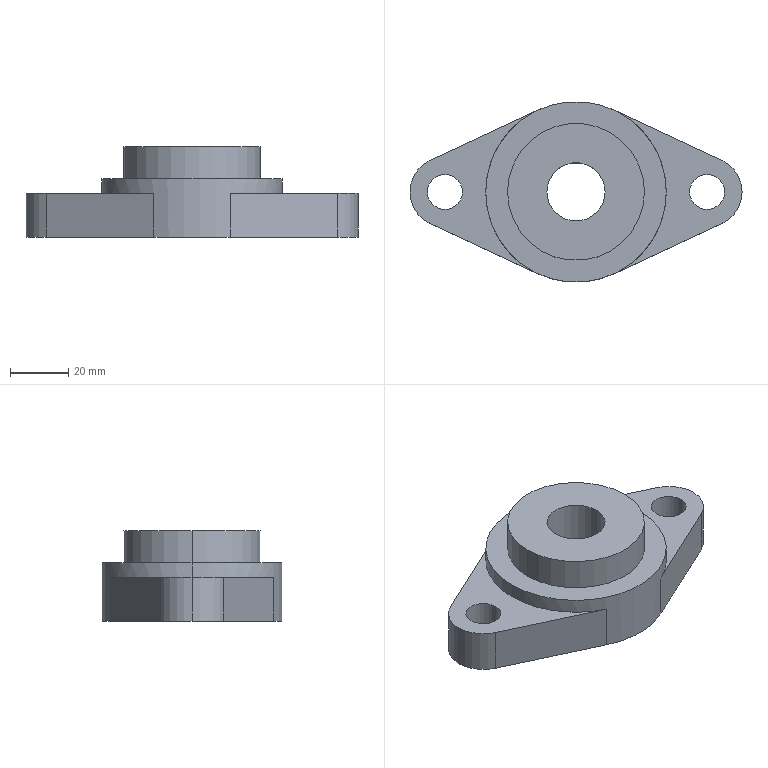Part | STEP file | Bearing housing 2 | 1 solid | 22 faces | box 114 x 62 x 31 mm | volume 91139 mm3 | cylinder 13 | plane 9 | commonest cylinder face diameters 12 x4 24 x3 20 x2 47 x2 62 x2
STEP:
#1=CARTESIAN_POINT('',(-89.013,-0.9655,15.));
#2=VERTEX_POINT('',#1);
#3=CARTESIAN_POINT('',(-101.013,-0.9655,15.));
#4=VERTEX_POINT('',#3);
#5=CARTESIAN_POINT('',(-95.013,-0.9655,15.));
#6=DIRECTION('',(0.,0.,-1.));
#7=DIRECTION('',(-1.,0.,0.));
#8=AXIS2_PLACEMENT_3D('',#5,#6,#7);
#9=CIRCLE('',#8,6.);
#10=EDGE_CURVE('',#2,#4,#9,.T.);
#11=ORIENTED_EDGE('',*,*,#10,.F.);
#12=CARTESIAN_POINT('',(-89.013,-0.9655,0.));
#13=VERTEX_POINT('',#12);
#14=CARTESIAN_POINT('',(-89.013,-0.9655,15.));
#15=DIRECTION('',(0.,0.,-1.));
#16=VECTOR('',#15,1000.);
#17=LINE('',#14,#16);
#18=EDGE_CURVE('',#2,#13,#17,.T.);
#19=ORIENTED_EDGE('',*,*,#18,.T.);
#20=CARTESIAN_POINT('',(-101.013,-0.9655,0.));
#21=VERTEX_POINT('',#20);
#22=CARTESIAN_POINT('',(-95.013,-0.9655,0.));
#23=DIRECTION('',(0.,0.,-1.));
#24=DIRECTION('',(-1.,0.,0.));
#25=AXIS2_PLACEMENT_3D('',#22,#23,#24);
#26=CIRCLE('',#25,6.);
#27=EDGE_CURVE('',#13,#21,#26,.T.);
#28=ORIENTED_EDGE('',*,*,#27,.T.);
#29=CARTESIAN_POINT('',(-101.013,-0.9655,15.));
#30=DIRECTION('',(0.,0.,-1.));
#31=VECTOR('',#30,1000.);
#32=LINE('',#29,#31);
#33=EDGE_CURVE('',#4,#21,#32,.T.);
#34=ORIENTED_EDGE('',*,*,#33,.F.);
#35=EDGE_LOOP('',(#11,#19,#28,#34));
#36=FACE_OUTER_BOUND('',#35,.T.);
#37=CARTESIAN_POINT('',(-95.013,-0.9655,15.));
#38=DIRECTION('',(0.,0.,-1.));
#39=DIRECTION('',(-1.,0.,0.));
#40=AXIS2_PLACEMENT_3D('',#37,#38,#39);
#41=CYLINDRICAL_SURFACE('',#40,6.);
#42=ADVANCED_FACE('',(#36),#41,.F.);
#43=CARTESIAN_POINT('',(-81.013,-0.9655,20.));
#44=VERTEX_POINT('',#43);
#45=CARTESIAN_POINT('',(-19.013,-0.9655,20.));
#46=VERTEX_POINT('',#45);
#47=CARTESIAN_POINT('',(-50.013,-0.9655,20.));
#48=DIRECTION('',(0.,0.,-1.));
#49=DIRECTION('',(-1.,0.,0.));
#50=AXIS2_PLACEMENT_3D('',#47,#48,#49);
#51=CIRCLE('',#50,31.);
#52=EDGE_CURVE('',#44,#46,#51,.T.);
#53=ORIENTED_EDGE('',*,*,#52,.T.);
#54=CARTESIAN_POINT('',(-19.013,-0.9655,15.));
#55=VERTEX_POINT('',#54);
#56=CARTESIAN_POINT('',(-19.013,-0.9655,15.));
#57=DIRECTION('',(0.,0.,-1.));
#58=VECTOR('',#57,1000.);
#59=LINE('',#56,#58);
#60=EDGE_CURVE('',#46,#55,#59,.T.);
#61=ORIENTED_EDGE('',*,*,#60,.T.);
#62=CARTESIAN_POINT('',(-36.924,27.136,15.));
#63=VERTEX_POINT('',#62);
#64=CARTESIAN_POINT('',(-50.013,-0.9655,15.));
#65=DIRECTION('',(0.,0.,1.));
#66=DIRECTION('',(-1.,0.,0.));
#67=AXIS2_PLACEMENT_3D('',#64,#65,#66);
#68=CIRCLE('',#67,31.);
#69=EDGE_CURVE('',#55,#63,#68,.T.);
#70=ORIENTED_EDGE('',*,*,#69,.T.);
#71=CARTESIAN_POINT('',(-36.924,27.136,0.));
#72=VERTEX_POINT('',#71);
#73=CARTESIAN_POINT('',(-36.924,27.136,15.));
#74=DIRECTION('',(0.,0.,-1.));
#75=VECTOR('',#74,1000.);
#76=LINE('',#73,#75);
#77=EDGE_CURVE('',#63,#72,#76,.T.);
#78=ORIENTED_EDGE('',*,*,#77,.T.);
#79=CARTESIAN_POINT('',(-63.102,27.136,0.));
#80=VERTEX_POINT('',#79);
#81=CARTESIAN_POINT('',(-50.013,-0.9655,0.));
#82=DIRECTION('',(0.,0.,1.));
#83=DIRECTION('',(-1.,0.,0.));
#84=AXIS2_PLACEMENT_3D('',#81,#82,#83);
#85=CIRCLE('',#84,31.);
#86=EDGE_CURVE('',#72,#80,#85,.T.);
#87=ORIENTED_EDGE('',*,*,#86,.T.);
#88=CARTESIAN_POINT('',(-63.102,27.136,15.));
#89=VERTEX_POINT('',#88);
#90=CARTESIAN_POINT('',(-63.102,27.136,15.));
#91=DIRECTION('',(0.,0.,1.));
#92=VECTOR('',#91,1000.);
#93=LINE('',#90,#92);
#94=EDGE_CURVE('',#80,#89,#93,.T.);
#95=ORIENTED_EDGE('',*,*,#94,.T.);
#96=CARTESIAN_POINT('',(-81.013,-0.9655,15.));
#97=VERTEX_POINT('',#96);
#98=CARTESIAN_POINT('',(-50.013,-0.9655,15.));
#99=DIRECTION('',(0.,0.,1.));
#100=DIRECTION('',(-1.,0.,0.));
#101=AXIS2_PLACEMENT_3D('',#98,#99,#100);
#102=CIRCLE('',#101,31.);
#103=EDGE_CURVE('',#89,#97,#102,.T.);
#104=ORIENTED_EDGE('',*,*,#103,.T.);
#105=CARTESIAN_POINT('',(-81.013,-0.9655,15.));
#106=DIRECTION('',(0.,0.,-1.));
#107=VECTOR('',#106,1000.);
#108=LINE('',#105,#107);
#109=EDGE_CURVE('',#44,#97,#108,.T.);
#110=ORIENTED_EDGE('',*,*,#109,.F.);
#111=EDGE_LOOP('',(#53,#61,#70,#78,#87,#95,#104,#110));
#112=FACE_OUTER_BOUND('',#111,.T.);
#113=CARTESIAN_POINT('',(-50.013,-0.9655,15.));
#114=DIRECTION('',(0.,0.,-1.));
#115=DIRECTION('',(-1.,0.,0.));
#116=AXIS2_PLACEMENT_3D('',#113,#114,#115);
#117=CYLINDRICAL_SURFACE('',#116,31.);
#118=ADVANCED_FACE('',(#112),#117,.T.);
#119=CARTESIAN_POINT('',(-100.08,-11.843,15.));
#120=VERTEX_POINT('',#119);
#121=CARTESIAN_POINT('',(-107.013,-0.9655,15.));
#122=VERTEX_POINT('',#121);
#123=CARTESIAN_POINT('',(-95.013,-0.9655,15.));
#124=DIRECTION('',(0.,0.,-1.));
#125=DIRECTION('',(-1.,0.,0.));
#126=AXIS2_PLACEMENT_3D('',#123,#124,#125);
#127=CIRCLE('',#126,12.);
#128=EDGE_CURVE('',#120,#122,#127,.T.);
#129=ORIENTED_EDGE('',*,*,#128,.T.);
#130=CARTESIAN_POINT('',(-107.013,-0.9655,0.));
#131=VERTEX_POINT('',#130);
#132=CARTESIAN_POINT('',(-107.013,-0.9655,15.));
#133=DIRECTION('',(0.,0.,-1.));
#134=VECTOR('',#133,1000.);
#135=LINE('',#132,#134);
#136=EDGE_CURVE('',#122,#131,#135,.T.);
#137=ORIENTED_EDGE('',*,*,#136,.T.);
#138=CARTESIAN_POINT('',(-100.08,-11.843,0.));
#139=VERTEX_POINT('',#138);
#140=CARTESIAN_POINT('',(-95.013,-0.9655,0.));
#141=DIRECTION('',(0.,0.,1.));
#142=DIRECTION('',(-1.,0.,0.));
#143=AXIS2_PLACEMENT_3D('',#140,#141,#142);
#144=CIRCLE('',#143,12.);
#145=EDGE_CURVE('',#131,#139,#144,.T.);
#146=ORIENTED_EDGE('',*,*,#145,.T.);
#147=CARTESIAN_POINT('',(-100.08,-11.843,15.));
#148=DIRECTION('',(0.,0.,1.));
#149=VECTOR('',#148,1000.);
#150=LINE('',#147,#149);
#151=EDGE_CURVE('',#139,#120,#150,.T.);
#152=ORIENTED_EDGE('',*,*,#151,.T.);
#153=EDGE_LOOP('',(#129,#137,#146,#152));
#154=FACE_OUTER_BOUND('',#153,.T.);
#155=CARTESIAN_POINT('',(-95.013,-0.9655,15.));
#156=DIRECTION('',(0.,0.,-1.));
#157=DIRECTION('',(-1.,0.,0.));
#158=AXIS2_PLACEMENT_3D('',#155,#156,#157);
#159=CYLINDRICAL_SURFACE('',#158,12.);
#160=ADVANCED_FACE('',(#154),#159,.T.);
#161=CARTESIAN_POINT('',(0.987,-0.9655,15.));
#162=VERTEX_POINT('',#161);
#163=CARTESIAN_POINT('',(-11.013,-0.9655,15.));
#164=VERTEX_POINT('',#163);
#165=CARTESIAN_POINT('',(-5.013,-0.9655,15.));
#166=DIRECTION('',(0.,0.,-1.));
#167=DIRECTION('',(-1.,0.,0.));
#168=AXIS2_PLACEMENT_3D('',#165,#166,#167);
#169=CIRCLE('',#168,6.);
#170=EDGE_CURVE('',#162,#164,#169,.T.);
#171=ORIENTED_EDGE('',*,*,#170,.F.);
#172=CARTESIAN_POINT('',(0.987,-0.9655,0.));
#173=VERTEX_POINT('',#172);
#174=CARTESIAN_POINT('',(0.987,-0.9655,15.));
#175=DIRECTION('',(0.,0.,-1.));
#176=VECTOR('',#175,1000.);
#177=LINE('',#174,#176);
#178=EDGE_CURVE('',#162,#173,#177,.T.);
#179=ORIENTED_EDGE('',*,*,#178,.T.);
#180=CARTESIAN_POINT('',(-11.013,-0.9655,0.));
#181=VERTEX_POINT('',#180);
#182=CARTESIAN_POINT('',(-5.013,-0.9655,0.));
#183=DIRECTION('',(0.,0.,-1.));
#184=DIRECTION('',(-1.,0.,0.));
#185=AXIS2_PLACEMENT_3D('',#182,#183,#184);
#186=CIRCLE('',#185,6.);
#187=EDGE_CURVE('',#173,#181,#186,.T.);
#188=ORIENTED_EDGE('',*,*,#187,.T.);
#189=CARTESIAN_POINT('',(-11.013,-0.9655,15.));
#190=DIRECTION('',(0.,0.,-1.));
#191=VECTOR('',#190,1000.);
#192=LINE('',#189,#191);
#193=EDGE_CURVE('',#164,#181,#192,.T.);
#194=ORIENTED_EDGE('',*,*,#193,.F.);
#195=EDGE_LOOP('',(#171,#179,#188,#194));
#196=FACE_OUTER_BOUND('',#195,.T.);
#197=CARTESIAN_POINT('',(-5.013,-0.9655,15.));
#198=DIRECTION('',(0.,0.,-1.));
#199=DIRECTION('',(-1.,0.,0.));
#200=AXIS2_PLACEMENT_3D('',#197,#198,#199);
#201=CYLINDRICAL_SURFACE('',#200,6.);
#202=ADVANCED_FACE('',(#196),#201,.F.);
#203=CARTESIAN_POINT('',(-40.013,-0.9655,0.));
#204=VERTEX_POINT('',#203);
#205=CARTESIAN_POINT('',(-60.013,-0.9655,0.));
#206=VERTEX_POINT('',#205);
#207=CARTESIAN_POINT('',(-50.013,-0.9655,0.));
#208=DIRECTION('',(0.,0.,-1.));
#209=DIRECTION('',(1.,0.,0.));
#210=AXIS2_PLACEMENT_3D('',#207,#208,#209);
#211=CIRCLE('',#210,10.);
#212=EDGE_CURVE('',#204,#206,#211,.T.);
#213=ORIENTED_EDGE('',*,*,#212,.T.);
#214=CARTESIAN_POINT('',(-60.013,-0.9655,31.));
#215=VERTEX_POINT('',#214);
#216=CARTESIAN_POINT('',(-60.013,-0.9655,-0.000025));
#217=DIRECTION('',(0.,0.,1.));
#218=VECTOR('',#217,1000.);
#219=LINE('',#216,#218);
#220=EDGE_CURVE('',#206,#215,#219,.T.);
#221=ORIENTED_EDGE('',*,*,#220,.T.);
#222=CARTESIAN_POINT('',(-40.013,-0.9655,31.));
#223=VERTEX_POINT('',#222);
#224=CARTESIAN_POINT('',(-50.013,-0.9655,31.));
#225=DIRECTION('',(0.,0.,-1.));
#226=DIRECTION('',(1.,0.,0.));
#227=AXIS2_PLACEMENT_3D('',#224,#225,#226);
#228=CIRCLE('',#227,10.);
#229=EDGE_CURVE('',#223,#215,#228,.T.);
#230=ORIENTED_EDGE('',*,*,#229,.F.);
#231=CARTESIAN_POINT('',(-40.013,-0.9655,-0.000025));
#232=DIRECTION('',(0.,0.,1.));
#233=VECTOR('',#232,1000.);
#234=LINE('',#231,#233);
#235=EDGE_CURVE('',#204,#223,#234,.T.);
#236=ORIENTED_EDGE('',*,*,#235,.F.);
#237=EDGE_LOOP('',(#213,#221,#230,#236));
#238=FACE_OUTER_BOUND('',#237,.T.);
#239=CARTESIAN_POINT('',(-50.013,-0.9655,-0.000025));
#240=DIRECTION('',(0.,0.,1.));
#241=DIRECTION('',(1.,0.,0.));
#242=AXIS2_PLACEMENT_3D('',#239,#240,#241);
#243=CYLINDRICAL_SURFACE('',#242,10.);
#244=ADVANCED_FACE('',(#238),#243,.F.);
#245=CARTESIAN_POINT('',(-26.513,-0.9655,31.));
#246=VERTEX_POINT('',#245);
#247=CARTESIAN_POINT('',(-73.513,-0.9655,31.));
#248=VERTEX_POINT('',#247);
#249=CARTESIAN_POINT('',(-50.013,-0.9655,31.));
#250=DIRECTION('',(0.,0.,1.));
#251=DIRECTION('',(-1.,0.,0.));
#252=AXIS2_PLACEMENT_3D('',#249,#250,#251);
#253=CIRCLE('',#252,23.5);
#254=EDGE_CURVE('',#246,#248,#253,.T.);
#255=ORIENTED_EDGE('',*,*,#254,.F.);
#256=CARTESIAN_POINT('',(-26.513,-0.9655,20.));
#257=VERTEX_POINT('',#256);
#258=CARTESIAN_POINT('',(-26.513,-0.9655,31.));
#259=DIRECTION('',(0.,0.,-1.));
#260=VECTOR('',#259,1000.);
#261=LINE('',#258,#260);
#262=EDGE_CURVE('',#246,#257,#261,.T.);
#263=ORIENTED_EDGE('',*,*,#262,.T.);
#264=CARTESIAN_POINT('',(-73.513,-0.9655,20.));
#265=VERTEX_POINT('',#264);
#266=CARTESIAN_POINT('',(-50.013,-0.9655,20.));
#267=DIRECTION('',(0.,0.,-1.));
#268=DIRECTION('',(-1.,0.,0.));
#269=AXIS2_PLACEMENT_3D('',#266,#267,#268);
#270=CIRCLE('',#269,23.5);
#271=EDGE_CURVE('',#265,#257,#270,.T.);
#272=ORIENTED_EDGE('',*,*,#271,.F.);
#273=CARTESIAN_POINT('',(-73.513,-0.9655,31.));
#274=DIRECTION('',(0.,0.,-1.));
#275=VECTOR('',#274,1000.);
#276=LINE('',#273,#275);
#277=EDGE_CURVE('',#248,#265,#276,.T.);
#278=ORIENTED_EDGE('',*,*,#277,.F.);
#279=EDGE_LOOP('',(#255,#263,#272,#278));
#280=FACE_OUTER_BOUND('',#279,.T.);
#281=CARTESIAN_POINT('',(-50.013,-0.9655,31.));
#282=DIRECTION('',(0.,0.,-1.));
#283=DIRECTION('',(-1.,0.,0.));
#284=AXIS2_PLACEMENT_3D('',#281,#282,#283);
#285=CYLINDRICAL_SURFACE('',#284,23.5);
#286=ADVANCED_FACE('',(#280),#285,.T.);
#287=CARTESIAN_POINT('',(-95.013,-0.9655,0.));
#288=DIRECTION('',(0.,0.,-1.));
#289=DIRECTION('',(-1.,0.,0.));
#290=AXIS2_PLACEMENT_3D('',#287,#288,#289);
#291=CIRCLE('',#290,6.);
#292=EDGE_CURVE('',#21,#13,#291,.T.);
#293=ORIENTED_EDGE('',*,*,#292,.F.);
#294=ORIENTED_EDGE('',*,*,#27,.F.);
#295=EDGE_LOOP('',(#293,#294));
#296=FACE_BOUND('',#295,.T.);
#297=CARTESIAN_POINT('',(0.05366,9.912,0.));
#298=VERTEX_POINT('',#297);
#299=CARTESIAN_POINT('',(0.05366,9.912,0.));
#300=DIRECTION('',(-0.9065,0.4222,0.));
#301=VECTOR('',#300,1000.);
#302=LINE('',#299,#301);
#303=EDGE_CURVE('',#298,#72,#302,.T.);
#304=ORIENTED_EDGE('',*,*,#303,.F.);
#305=CARTESIAN_POINT('',(0.05366,-11.843,0.));
#306=VERTEX_POINT('',#305);
#307=CARTESIAN_POINT('',(-5.013,-0.9655,0.));
#308=DIRECTION('',(0.,0.,1.));
#309=DIRECTION('',(-1.,0.,0.));
#310=AXIS2_PLACEMENT_3D('',#307,#308,#309);
#311=CIRCLE('',#310,12.);
#312=EDGE_CURVE('',#306,#298,#311,.T.);
#313=ORIENTED_EDGE('',*,*,#312,.F.);
#314=CARTESIAN_POINT('',(-36.924,-29.067,0.));
#315=VERTEX_POINT('',#314);
#316=CARTESIAN_POINT('',(-36.924,-29.067,0.));
#317=DIRECTION('',(0.9065,0.4222,0.));
#318=VECTOR('',#317,1000.);
#319=LINE('',#316,#318);
#320=EDGE_CURVE('',#315,#306,#319,.T.);
#321=ORIENTED_EDGE('',*,*,#320,.F.);
#322=CARTESIAN_POINT('',(-63.102,-29.067,0.));
#323=VERTEX_POINT('',#322);
#324=CARTESIAN_POINT('',(-50.013,-0.9655,0.));
#325=DIRECTION('',(0.,0.,1.));
#326=DIRECTION('',(-1.,0.,0.));
#327=AXIS2_PLACEMENT_3D('',#324,#325,#326);
#328=CIRCLE('',#327,31.);
#329=EDGE_CURVE('',#323,#315,#328,.T.);
#330=ORIENTED_EDGE('',*,*,#329,.F.);
#331=CARTESIAN_POINT('',(-100.08,-11.843,0.));
#332=DIRECTION('',(0.9065,-0.4222,0.));
#333=VECTOR('',#332,1000.);
#334=LINE('',#331,#333);
#335=EDGE_CURVE('',#139,#323,#334,.T.);
#336=ORIENTED_EDGE('',*,*,#335,.F.);
#337=ORIENTED_EDGE('',*,*,#145,.F.);
#338=CARTESIAN_POINT('',(-100.08,9.912,0.));
#339=VERTEX_POINT('',#338);
#340=CARTESIAN_POINT('',(-95.013,-0.9655,0.));
#341=DIRECTION('',(0.,0.,1.));
#342=DIRECTION('',(-1.,0.,0.));
#343=AXIS2_PLACEMENT_3D('',#340,#341,#342);
#344=CIRCLE('',#343,12.);
#345=EDGE_CURVE('',#339,#131,#344,.T.);
#346=ORIENTED_EDGE('',*,*,#345,.F.);
#347=CARTESIAN_POINT('',(-63.102,27.136,0.));
#348=DIRECTION('',(-0.9065,-0.4222,0.));
#349=VECTOR('',#348,1000.);
#350=LINE('',#347,#349);
#351=EDGE_CURVE('',#80,#339,#350,.T.);
#352=ORIENTED_EDGE('',*,*,#351,.F.);
#353=ORIENTED_EDGE('',*,*,#86,.F.);
#354=EDGE_LOOP('',(#304,#313,#321,#330,#336,#337,#346,#352,#353));
#355=FACE_OUTER_BOUND('',#354,.T.);
#356=CARTESIAN_POINT('',(-5.013,-0.9655,0.));
#357=DIRECTION('',(0.,0.,-1.));
#358=DIRECTION('',(-1.,0.,0.));
#359=AXIS2_PLACEMENT_3D('',#356,#357,#358);
#360=CIRCLE('',#359,6.);
#361=EDGE_CURVE('',#181,#173,#360,.T.);
#362=ORIENTED_EDGE('',*,*,#361,.F.);
#363=ORIENTED_EDGE('',*,*,#187,.F.);
#364=EDGE_LOOP('',(#362,#363));
#365=FACE_BOUND('',#364,.T.);
#366=ORIENTED_EDGE('',*,*,#212,.F.);
#367=CARTESIAN_POINT('',(-50.013,-0.9655,0.));
#368=DIRECTION('',(0.,0.,-1.));
#369=DIRECTION('',(1.,0.,0.));
#370=AXIS2_PLACEMENT_3D('',#367,#368,#369);
#371=CIRCLE('',#370,10.);
#372=EDGE_CURVE('',#206,#204,#371,.T.);
#373=ORIENTED_EDGE('',*,*,#372,.F.);
#374=EDGE_LOOP('',(#366,#373));
#375=FACE_BOUND('',#374,.T.);
#376=CARTESIAN_POINT('',(-50.013,-0.9655,0.));
#377=DIRECTION('',(0.,0.,1.));
#378=DIRECTION('',(1.,0.,0.));
#379=AXIS2_PLACEMENT_3D('',#376,#377,#378);
#380=PLANE('',#379);
#381=ADVANCED_FACE('',(#296,#355,#365,#375),#380,.F.);
#382=ORIENTED_EDGE('',*,*,#18,.F.);
#383=CARTESIAN_POINT('',(-95.013,-0.9655,15.));
#384=DIRECTION('',(0.,0.,-1.));
#385=DIRECTION('',(-1.,0.,0.));
#386=AXIS2_PLACEMENT_3D('',#383,#384,#385);
#387=CIRCLE('',#386,6.);
#388=EDGE_CURVE('',#4,#2,#387,.T.);
#389=ORIENTED_EDGE('',*,*,#388,.F.);
#390=ORIENTED_EDGE('',*,*,#33,.T.);
#391=ORIENTED_EDGE('',*,*,#292,.T.);
#392=EDGE_LOOP('',(#382,#389,#390,#391));
#393=FACE_OUTER_BOUND('',#392,.T.);
#394=CARTESIAN_POINT('',(-95.013,-0.9655,15.));
#395=DIRECTION('',(0.,0.,-1.));
#396=DIRECTION('',(-1.,0.,0.));
#397=AXIS2_PLACEMENT_3D('',#394,#395,#396);
#398=CYLINDRICAL_SURFACE('',#397,6.);
#399=ADVANCED_FACE('',(#393),#398,.F.);
#400=ORIENTED_EDGE('',*,*,#60,.F.);
#401=CARTESIAN_POINT('',(-50.013,-0.9655,20.));
#402=DIRECTION('',(0.,0.,-1.));
#403=DIRECTION('',(-1.,0.,0.));
#404=AXIS2_PLACEMENT_3D('',#401,#402,#403);
#405=CIRCLE('',#404,31.);
#406=EDGE_CURVE('',#46,#44,#405,.T.);
#407=ORIENTED_EDGE('',*,*,#406,.T.);
#408=ORIENTED_EDGE('',*,*,#109,.T.);
#409=CARTESIAN_POINT('',(-63.102,-29.067,15.));
#410=VERTEX_POINT('',#409);
#411=CARTESIAN_POINT('',(-50.013,-0.9655,15.));
#412=DIRECTION('',(0.,0.,1.));
#413=DIRECTION('',(-1.,0.,0.));
#414=AXIS2_PLACEMENT_3D('',#411,#412,#413);
#415=CIRCLE('',#414,31.);
#416=EDGE_CURVE('',#97,#410,#415,.T.);
#417=ORIENTED_EDGE('',*,*,#416,.T.);
#418=CARTESIAN_POINT('',(-63.102,-29.067,15.));
#419=DIRECTION('',(0.,0.,-1.));
#420=VECTOR('',#419,1000.);
#421=LINE('',#418,#420);
#422=EDGE_CURVE('',#410,#323,#421,.T.);
#423=ORIENTED_EDGE('',*,*,#422,.T.);
#424=ORIENTED_EDGE('',*,*,#329,.T.);
#425=CARTESIAN_POINT('',(-36.924,-29.067,15.));
#426=VERTEX_POINT('',#425);
#427=CARTESIAN_POINT('',(-36.924,-29.067,15.));
#428=DIRECTION('',(0.,0.,1.));
#429=VECTOR('',#428,1000.);
#430=LINE('',#427,#429);
#431=EDGE_CURVE('',#315,#426,#430,.T.);
#432=ORIENTED_EDGE('',*,*,#431,.T.);
#433=CARTESIAN_POINT('',(-50.013,-0.9655,15.));
#434=DIRECTION('',(0.,0.,1.));
#435=DIRECTION('',(-1.,0.,0.));
#436=AXIS2_PLACEMENT_3D('',#433,#434,#435);
#437=CIRCLE('',#436,31.);
#438=EDGE_CURVE('',#426,#55,#437,.T.);
#439=ORIENTED_EDGE('',*,*,#438,.T.);
#440=EDGE_LOOP('',(#400,#407,#408,#417,#423,#424,#432,#439));
#441=FACE_OUTER_BOUND('',#440,.T.);
#442=CARTESIAN_POINT('',(-50.013,-0.9655,15.));
#443=DIRECTION('',(0.,0.,-1.));
#444=DIRECTION('',(-1.,0.,0.));
#445=AXIS2_PLACEMENT_3D('',#442,#443,#444);
#446=CYLINDRICAL_SURFACE('',#445,31.);
#447=ADVANCED_FACE('',(#441),#446,.T.);
#448=ORIENTED_EDGE('',*,*,#77,.F.);
#449=CARTESIAN_POINT('',(0.05366,9.912,15.));
#450=VERTEX_POINT('',#449);
#451=CARTESIAN_POINT('',(-36.924,27.136,15.));
#452=DIRECTION('',(-0.9065,0.4222,0.));
#453=VECTOR('',#452,1000.);
#454=LINE('',#451,#453);
#455=EDGE_CURVE('',#450,#63,#454,.T.);
#456=ORIENTED_EDGE('',*,*,#455,.F.);
#457=CARTESIAN_POINT('',(0.05366,9.912,15.));
#458=DIRECTION('',(0.,0.,1.));
#459=VECTOR('',#458,1000.);
#460=LINE('',#457,#459);
#461=EDGE_CURVE('',#298,#450,#460,.T.);
#462=ORIENTED_EDGE('',*,*,#461,.F.);
#463=ORIENTED_EDGE('',*,*,#303,.T.);
#464=EDGE_LOOP('',(#448,#456,#462,#463));
#465=FACE_OUTER_BOUND('',#464,.T.);
#466=CARTESIAN_POINT('',(-36.924,27.136,15.));
#467=DIRECTION('',(-0.4222,-0.9065,0.));
#468=DIRECTION('',(0.9065,-0.4222,0.));
#469=AXIS2_PLACEMENT_3D('',#466,#467,#468);
#470=PLANE('',#469);
#471=ADVANCED_FACE('',(#465),#470,.F.);
#472=CARTESIAN_POINT('',(0.05366,-11.843,15.));
#473=VERTEX_POINT('',#472);
#474=CARTESIAN_POINT('',(-5.013,-0.9655,15.));
#475=DIRECTION('',(0.,0.,-1.));
#476=DIRECTION('',(-1.,0.,0.));
#477=AXIS2_PLACEMENT_3D('',#474,#475,#476);
#478=CIRCLE('',#477,12.);
#479=EDGE_CURVE('',#450,#473,#478,.T.);
#480=ORIENTED_EDGE('',*,*,#479,.T.);
#481=CARTESIAN_POINT('',(0.05366,-11.843,15.));
#482=DIRECTION('',(0.,0.,-1.));
#483=VECTOR('',#482,1000.);
#484=LINE('',#481,#483);
#485=EDGE_CURVE('',#473,#306,#484,.T.);
#486=ORIENTED_EDGE('',*,*,#485,.T.);
#487=ORIENTED_EDGE('',*,*,#312,.T.);
#488=ORIENTED_EDGE('',*,*,#461,.T.);
#489=EDGE_LOOP('',(#480,#486,#487,#488));
#490=FACE_OUTER_BOUND('',#489,.T.);
#491=CARTESIAN_POINT('',(-5.013,-0.9655,15.));
#492=DIRECTION('',(0.,0.,-1.));
#493=DIRECTION('',(-1.,0.,0.));
#494=AXIS2_PLACEMENT_3D('',#491,#492,#493);
#495=CYLINDRICAL_SURFACE('',#494,12.);
#496=ADVANCED_FACE('',(#490),#495,.T.);
#497=ORIENTED_EDGE('',*,*,#485,.F.);
#498=CARTESIAN_POINT('',(-36.924,-29.067,15.));
#499=DIRECTION('',(0.9065,0.4222,0.));
#500=VECTOR('',#499,1000.);
#501=LINE('',#498,#500);
#502=EDGE_CURVE('',#426,#473,#501,.T.);
#503=ORIENTED_EDGE('',*,*,#502,.F.);
#504=ORIENTED_EDGE('',*,*,#431,.F.);
#505=ORIENTED_EDGE('',*,*,#320,.T.);
#506=EDGE_LOOP('',(#497,#503,#504,#505));
#507=FACE_OUTER_BOUND('',#506,.T.);
#508=CARTESIAN_POINT('',(-36.924,-29.067,15.));
#509=DIRECTION('',(-0.4222,0.9065,0.));
#510=DIRECTION('',(-0.9065,-0.4222,0.));
#511=AXIS2_PLACEMENT_3D('',#508,#509,#510);
#512=PLANE('',#511);
#513=ADVANCED_FACE('',(#507),#512,.F.);
#514=ORIENTED_EDGE('',*,*,#422,.F.);
#515=CARTESIAN_POINT('',(-100.08,-11.843,15.));
#516=DIRECTION('',(0.9065,-0.4222,0.));
#517=VECTOR('',#516,1000.);
#518=LINE('',#515,#517);
#519=EDGE_CURVE('',#120,#410,#518,.T.);
#520=ORIENTED_EDGE('',*,*,#519,.F.);
#521=ORIENTED_EDGE('',*,*,#151,.F.);
#522=ORIENTED_EDGE('',*,*,#335,.T.);
#523=EDGE_LOOP('',(#514,#520,#521,#522));
#524=FACE_OUTER_BOUND('',#523,.T.);
#525=CARTESIAN_POINT('',(-100.08,-11.843,15.));
#526=DIRECTION('',(0.4222,0.9065,0.));
#527=DIRECTION('',(-0.9065,0.4222,0.));
#528=AXIS2_PLACEMENT_3D('',#525,#526,#527);
#529=PLANE('',#528);
#530=ADVANCED_FACE('',(#524),#529,.F.);
#531=ORIENTED_EDGE('',*,*,#136,.F.);
#532=CARTESIAN_POINT('',(-100.08,9.912,15.));
#533=VERTEX_POINT('',#532);
#534=CARTESIAN_POINT('',(-95.013,-0.9655,15.));
#535=DIRECTION('',(0.,0.,-1.));
#536=DIRECTION('',(-1.,0.,0.));
#537=AXIS2_PLACEMENT_3D('',#534,#535,#536);
#538=CIRCLE('',#537,12.);
#539=EDGE_CURVE('',#122,#533,#538,.T.);
#540=ORIENTED_EDGE('',*,*,#539,.T.);
#541=CARTESIAN_POINT('',(-100.08,9.912,15.));
#542=DIRECTION('',(0.,0.,-1.));
#543=VECTOR('',#542,1000.);
#544=LINE('',#541,#543);
#545=EDGE_CURVE('',#533,#339,#544,.T.);
#546=ORIENTED_EDGE('',*,*,#545,.T.);
#547=ORIENTED_EDGE('',*,*,#345,.T.);
#548=EDGE_LOOP('',(#531,#540,#546,#547));
#549=FACE_OUTER_BOUND('',#548,.T.);
#550=CARTESIAN_POINT('',(-95.013,-0.9655,15.));
#551=DIRECTION('',(0.,0.,-1.));
#552=DIRECTION('',(-1.,0.,0.));
#553=AXIS2_PLACEMENT_3D('',#550,#551,#552);
#554=CYLINDRICAL_SURFACE('',#553,12.);
#555=ADVANCED_FACE('',(#549),#554,.T.);
#556=ORIENTED_EDGE('',*,*,#545,.F.);
#557=CARTESIAN_POINT('',(-100.08,9.912,15.));
#558=DIRECTION('',(-0.9065,-0.4222,0.));
#559=VECTOR('',#558,1000.);
#560=LINE('',#557,#559);
#561=EDGE_CURVE('',#89,#533,#560,.T.);
#562=ORIENTED_EDGE('',*,*,#561,.F.);
#563=ORIENTED_EDGE('',*,*,#94,.F.);
#564=ORIENTED_EDGE('',*,*,#351,.T.);
#565=EDGE_LOOP('',(#556,#562,#563,#564));
#566=FACE_OUTER_BOUND('',#565,.T.);
#567=CARTESIAN_POINT('',(-100.08,9.912,15.));
#568=DIRECTION('',(0.4222,-0.9065,0.));
#569=DIRECTION('',(0.9065,0.4222,0.));
#570=AXIS2_PLACEMENT_3D('',#567,#568,#569);
#571=PLANE('',#570);
#572=ADVANCED_FACE('',(#566),#571,.F.);
#573=ORIENTED_EDGE('',*,*,#178,.F.);
#574=CARTESIAN_POINT('',(-5.013,-0.9655,15.));
#575=DIRECTION('',(0.,0.,-1.));
#576=DIRECTION('',(-1.,0.,0.));
#577=AXIS2_PLACEMENT_3D('',#574,#575,#576);
#578=CIRCLE('',#577,6.);
#579=EDGE_CURVE('',#164,#162,#578,.T.);
#580=ORIENTED_EDGE('',*,*,#579,.F.);
#581=ORIENTED_EDGE('',*,*,#193,.T.);
#582=ORIENTED_EDGE('',*,*,#361,.T.);
#583=EDGE_LOOP('',(#573,#580,#581,#582));
#584=FACE_OUTER_BOUND('',#583,.T.);
#585=CARTESIAN_POINT('',(-5.013,-0.9655,15.));
#586=DIRECTION('',(0.,0.,-1.));
#587=DIRECTION('',(-1.,0.,0.));
#588=AXIS2_PLACEMENT_3D('',#585,#586,#587);
#589=CYLINDRICAL_SURFACE('',#588,6.);
#590=ADVANCED_FACE('',(#584),#589,.F.);
#591=ORIENTED_EDGE('',*,*,#220,.F.);
#592=ORIENTED_EDGE('',*,*,#372,.T.);
#593=ORIENTED_EDGE('',*,*,#235,.T.);
#594=CARTESIAN_POINT('',(-50.013,-0.9655,31.));
#595=DIRECTION('',(0.,0.,-1.));
#596=DIRECTION('',(1.,0.,0.));
#597=AXIS2_PLACEMENT_3D('',#594,#595,#596);
#598=CIRCLE('',#597,10.);
#599=EDGE_CURVE('',#215,#223,#598,.T.);
#600=ORIENTED_EDGE('',*,*,#599,.F.);
#601=EDGE_LOOP('',(#591,#592,#593,#600));
#602=FACE_OUTER_BOUND('',#601,.T.);
#603=CARTESIAN_POINT('',(-50.013,-0.9655,-0.000025));
#604=DIRECTION('',(0.,0.,1.));
#605=DIRECTION('',(1.,0.,0.));
#606=AXIS2_PLACEMENT_3D('',#603,#604,#605);
#607=CYLINDRICAL_SURFACE('',#606,10.);
#608=ADVANCED_FACE('',(#602),#607,.F.);
#609=ORIENTED_EDGE('',*,*,#388,.T.);
#610=ORIENTED_EDGE('',*,*,#10,.T.);
#611=EDGE_LOOP('',(#609,#610));
#612=FACE_BOUND('',#611,.T.);
#613=ORIENTED_EDGE('',*,*,#519,.T.);
#614=ORIENTED_EDGE('',*,*,#416,.F.);
#615=ORIENTED_EDGE('',*,*,#103,.F.);
#616=ORIENTED_EDGE('',*,*,#561,.T.);
#617=ORIENTED_EDGE('',*,*,#539,.F.);
#618=ORIENTED_EDGE('',*,*,#128,.F.);
#619=EDGE_LOOP('',(#613,#614,#615,#616,#617,#618));
#620=FACE_OUTER_BOUND('',#619,.T.);
#621=CARTESIAN_POINT('',(-50.013,-0.9655,15.));
#622=DIRECTION('',(0.,0.,1.));
#623=DIRECTION('',(1.,0.,0.));
#624=AXIS2_PLACEMENT_3D('',#621,#622,#623);
#625=PLANE('',#624);
#626=ADVANCED_FACE('',(#612,#620),#625,.T.);
#627=ORIENTED_EDGE('',*,*,#579,.T.);
#628=ORIENTED_EDGE('',*,*,#170,.T.);
#629=EDGE_LOOP('',(#627,#628));
#630=FACE_BOUND('',#629,.T.);
#631=ORIENTED_EDGE('',*,*,#455,.T.);
#632=ORIENTED_EDGE('',*,*,#69,.F.);
#633=ORIENTED_EDGE('',*,*,#438,.F.);
#634=ORIENTED_EDGE('',*,*,#502,.T.);
#635=ORIENTED_EDGE('',*,*,#479,.F.);
#636=EDGE_LOOP('',(#631,#632,#633,#634,#635));
#637=FACE_OUTER_BOUND('',#636,.T.);
#638=CARTESIAN_POINT('',(-50.013,-0.9655,15.));
#639=DIRECTION('',(0.,0.,1.));
#640=DIRECTION('',(1.,0.,0.));
#641=AXIS2_PLACEMENT_3D('',#638,#639,#640);
#642=PLANE('',#641);
#643=ADVANCED_FACE('',(#630,#637),#642,.T.);
#644=ORIENTED_EDGE('',*,*,#271,.T.);
#645=CARTESIAN_POINT('',(-50.013,-0.9655,20.));
#646=DIRECTION('',(0.,0.,-1.));
#647=DIRECTION('',(-1.,0.,0.));
#648=AXIS2_PLACEMENT_3D('',#645,#646,#647);
#649=CIRCLE('',#648,23.5);
#650=EDGE_CURVE('',#257,#265,#649,.T.);
#651=ORIENTED_EDGE('',*,*,#650,.T.);
#652=EDGE_LOOP('',(#644,#651));
#653=FACE_BOUND('',#652,.T.);
#654=ORIENTED_EDGE('',*,*,#52,.F.);
#655=ORIENTED_EDGE('',*,*,#406,.F.);
#656=EDGE_LOOP('',(#654,#655));
#657=FACE_OUTER_BOUND('',#656,.T.);
#658=CARTESIAN_POINT('',(-50.013,-0.9655,20.));
#659=DIRECTION('',(0.,0.,1.));
#660=DIRECTION('',(1.,0.,0.));
#661=AXIS2_PLACEMENT_3D('',#658,#659,#660);
#662=PLANE('',#661);
#663=ADVANCED_FACE('',(#653,#657),#662,.T.);
#664=CARTESIAN_POINT('',(-50.013,-0.9655,31.));
#665=DIRECTION('',(0.,0.,1.));
#666=DIRECTION('',(-1.,0.,0.));
#667=AXIS2_PLACEMENT_3D('',#664,#665,#666);
#668=CIRCLE('',#667,23.5);
#669=EDGE_CURVE('',#248,#246,#668,.T.);
#670=ORIENTED_EDGE('',*,*,#669,.T.);
#671=ORIENTED_EDGE('',*,*,#254,.T.);
#672=EDGE_LOOP('',(#670,#671));
#673=FACE_OUTER_BOUND('',#672,.T.);
#674=ORIENTED_EDGE('',*,*,#229,.T.);
#675=ORIENTED_EDGE('',*,*,#599,.T.);
#676=EDGE_LOOP('',(#674,#675));
#677=FACE_BOUND('',#676,.T.);
#678=CARTESIAN_POINT('',(-50.013,-0.9655,31.));
#679=DIRECTION('',(0.,0.,1.));
#680=DIRECTION('',(1.,0.,0.));
#681=AXIS2_PLACEMENT_3D('',#678,#679,#680);
#682=PLANE('',#681);
#683=ADVANCED_FACE('',(#673,#677),#682,.T.);
#684=ORIENTED_EDGE('',*,*,#262,.F.);
#685=ORIENTED_EDGE('',*,*,#669,.F.);
#686=ORIENTED_EDGE('',*,*,#277,.T.);
#687=ORIENTED_EDGE('',*,*,#650,.F.);
#688=EDGE_LOOP('',(#684,#685,#686,#687));
#689=FACE_OUTER_BOUND('',#688,.T.);
#690=CARTESIAN_POINT('',(-50.013,-0.9655,31.));
#691=DIRECTION('',(0.,0.,-1.));
#692=DIRECTION('',(-1.,0.,0.));
#693=AXIS2_PLACEMENT_3D('',#690,#691,#692);
#694=CYLINDRICAL_SURFACE('',#693,23.5);
#695=ADVANCED_FACE('',(#689),#694,.T.);
#696=CLOSED_SHELL('',(#42,#118,#160,#202,#244,#286,#381,#399,#447,#471,#496,#513,#530,#555,#572,#590,#608,#626,#643,#663,#683,#695));
#697=MANIFOLD_SOLID_BREP('',#696);
#698=CARTESIAN_POINT('',(0.,0.,0.));
#699=DIRECTION('',(0.,0.,1.));
#700=DIRECTION('',(1.,0.,0.));
#701=AXIS2_PLACEMENT_3D('',#698,#699,#700);
#702=(LENGTH_UNIT()NAMED_UNIT(*)SI_UNIT(.MILLI.,.METRE.));
#703=UNCERTAINTY_MEASURE_WITH_UNIT(LENGTH_MEASURE(0.00001),#702,'','');
#704=(NAMED_UNIT(*)PLANE_ANGLE_UNIT()SI_UNIT($,.RADIAN.));
#705=(NAMED_UNIT(*)SI_UNIT($,.STERADIAN.)SOLID_ANGLE_UNIT());
#706=(GEOMETRIC_REPRESENTATION_CONTEXT(3)GLOBAL_UNCERTAINTY_ASSIGNED_CONTEXT((#703))GLOBAL_UNIT_ASSIGNED_CONTEXT((#702,#704,#705))REPRESENTATION_CONTEXT('',''));
#707=ADVANCED_BREP_SHAPE_REPRESENTATION('',(#697,#701),#706);